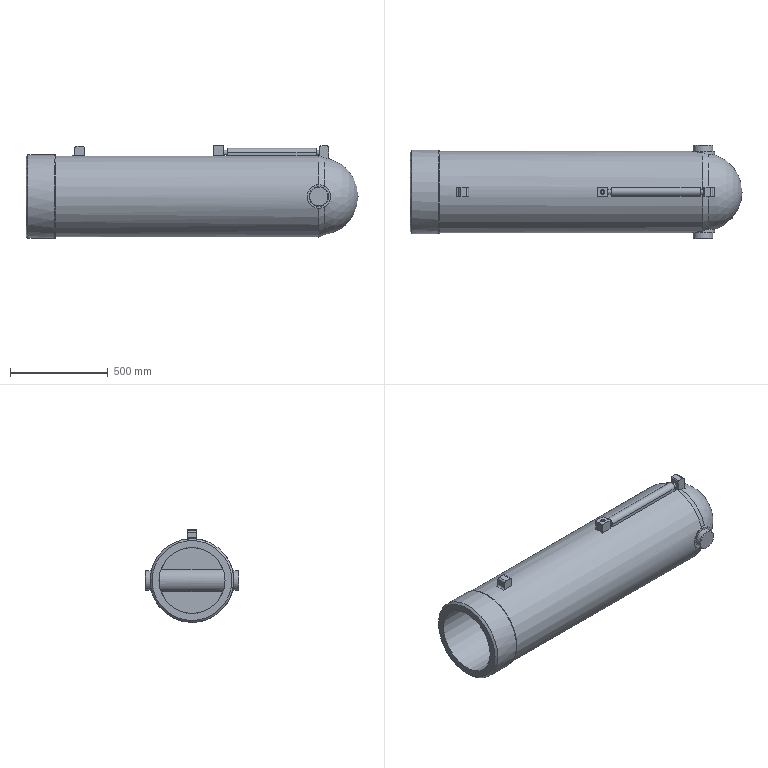Part | NX | features 立柱缸一级 2 | 1 solid | 56 faces | box 1697 x 478 x 474 mm | volume 93646895 mm3 | plane 29 | cylinder 18 | cone 5 | torus 3 | sphere 1 | commonest cylinder face diameters 20 x3 120 x3 24.6 x2 100 x2 10 x1 13.78 x1